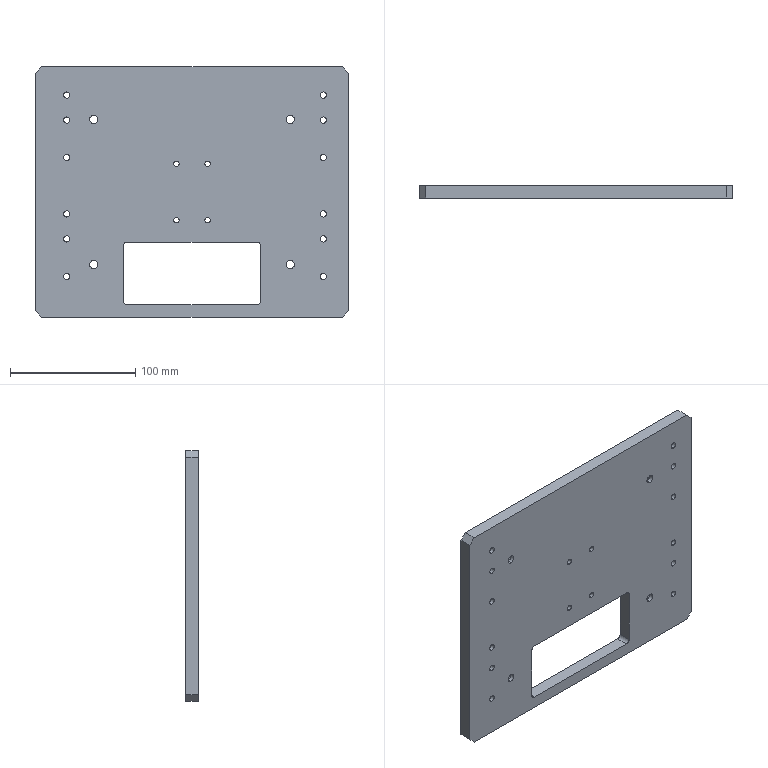Part | SolidWorks | features HoleWzd 3, Cut 2, Chamfer 1, Extrusion 1, Fillet 1 | 1 solid | 82 faces | box 250 x 10 x 200 mm | volume 437930 mm3 | cylinder 60 | plane 22 | commonest cylinder face diameters 5 x24 4.5 x8 6.6 x8 8 x8 11 x8 6 x4